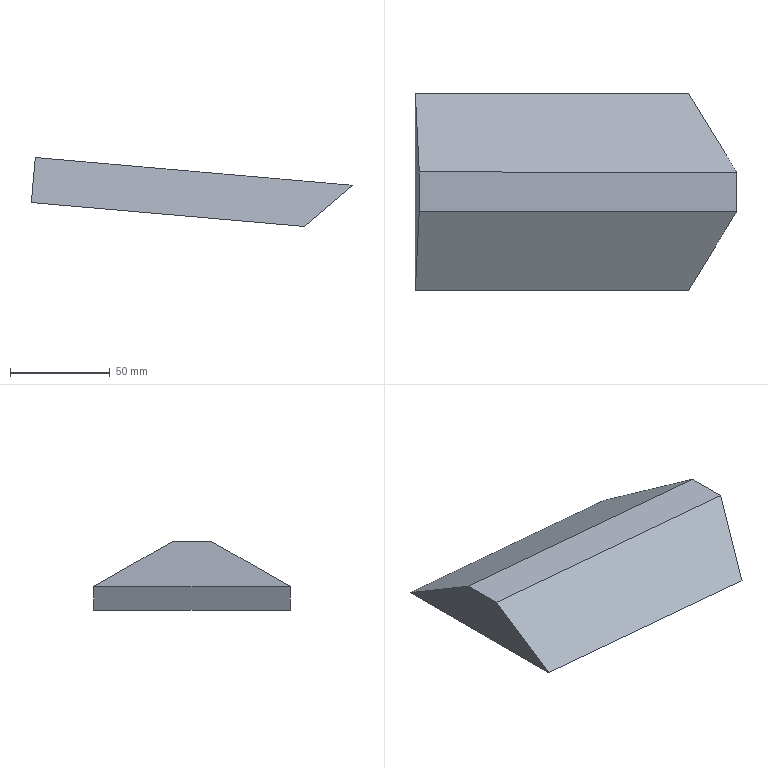Part | NX | features solid 2 | 1 solid | 6 faces | box 161.368 x 98.588 x 34.603 mm | volume 196929 mm3 | plane 6
STEP:
#1=CARTESIAN_POINT('',(-1040.,229.294,-200.));
#2=VERTEX_POINT('',#1);
#3=CARTESIAN_POINT('',(-1040.,130.706,-200.));
#4=VERTEX_POINT('',#3);
#5=CARTESIAN_POINT('',(-1040.,260.,-200.));
#6=DIRECTION('',(0.,-1.,0.));
#7=VECTOR('',#6,1000.);
#8=LINE('',#5,#7);
#9=EDGE_CURVE('',#2,#4,#8,.T.);
#10=ORIENTED_EDGE('',*,*,#9,.T.);
#11=CARTESIAN_POINT('',(-1038.023,170.,-177.4));
#12=VERTEX_POINT('',#11);
#13=CARTESIAN_POINT('',(-1041.545,100.,-217.661));
#14=DIRECTION('',(0.04358,0.866,0.4981));
#15=VECTOR('',#14,1000.);
#16=LINE('',#13,#15);
#17=EDGE_CURVE('',#4,#12,#16,.T.);
#18=ORIENTED_EDGE('',*,*,#17,.T.);
#19=CARTESIAN_POINT('',(-1038.023,190.,-177.4));
#20=VERTEX_POINT('',#19);
#21=CARTESIAN_POINT('',(-1038.023,260.,-177.4));
#22=DIRECTION('',(0.,-1.,0.));
#23=VECTOR('',#22,1000.);
#24=LINE('',#21,#23);
#25=EDGE_CURVE('',#20,#12,#24,.T.);
#26=ORIENTED_EDGE('',*,*,#25,.F.);
#27=CARTESIAN_POINT('',(-1041.545,260.,-217.661));
#28=DIRECTION('',(0.04358,-0.866,0.4981));
#29=VECTOR('',#28,1000.);
#30=LINE('',#27,#29);
#31=EDGE_CURVE('',#2,#20,#30,.T.);
#32=ORIENTED_EDGE('',*,*,#31,.F.);
#33=EDGE_LOOP('',(#10,#18,#26,#32));
#34=FACE_BOUND('',#33,.T.);
#35=CARTESIAN_POINT('',(-1038.023,260.,-177.4));
#36=DIRECTION('',(-0.9962,0.,0.08716));
#37=DIRECTION('',(-0.08716,0.,-0.9962));
#38=AXIS2_PLACEMENT_3D('',#35,#36,#37);
#39=PLANE('',#38);
#40=ADVANCED_FACE('',(#34),#39,.T.);
#41=CARTESIAN_POINT('',(-902.806,130.706,-212.003));
#42=VERTEX_POINT('',#41);
#43=CARTESIAN_POINT('',(-902.806,130.706,-212.003));
#44=DIRECTION('',(0.9962,0.,-0.08716));
#45=VECTOR('',#44,1000.);
#46=LINE('',#43,#45);
#47=EDGE_CURVE('',#4,#42,#46,.T.);
#48=ORIENTED_EDGE('',*,*,#47,.F.);
#49=ORIENTED_EDGE('',*,*,#9,.F.);
#50=CARTESIAN_POINT('',(-902.806,229.294,-212.003));
#51=VERTEX_POINT('',#50);
#52=CARTESIAN_POINT('',(-902.806,229.294,-212.003));
#53=DIRECTION('',(-0.9962,0.,0.08716));
#54=VECTOR('',#53,1000.);
#55=LINE('',#52,#54);
#56=EDGE_CURVE('',#51,#2,#55,.T.);
#57=ORIENTED_EDGE('',*,*,#56,.F.);
#58=CARTESIAN_POINT('',(-902.806,260.,-212.003));
#59=DIRECTION('',(0.,-1.,0.));
#60=VECTOR('',#59,1000.);
#61=LINE('',#58,#60);
#62=EDGE_CURVE('',#51,#42,#61,.T.);
#63=ORIENTED_EDGE('',*,*,#62,.T.);
#64=EDGE_LOOP('',(#48,#49,#57,#63));
#65=FACE_BOUND('',#64,.T.);
#66=CARTESIAN_POINT('',(-902.806,260.,-212.003));
#67=DIRECTION('',(0.08716,0.,0.9962));
#68=DIRECTION('',(-0.9962,0.,0.08716));
#69=AXIS2_PLACEMENT_3D('',#66,#67,#68);
#70=PLANE('',#69);
#71=ADVANCED_FACE('',(#65),#70,.F.);
#72=CARTESIAN_POINT('',(-878.632,170.,-191.345));
#73=VERTEX_POINT('',#72);
#74=CARTESIAN_POINT('',(-845.173,224.384,-162.753));
#75=DIRECTION('',(0.4782,0.7773,0.4087));
#76=VECTOR('',#75,1000.);
#77=LINE('',#74,#76);
#78=EDGE_CURVE('',#42,#73,#77,.T.);
#79=ORIENTED_EDGE('',*,*,#78,.F.);
#80=ORIENTED_EDGE('',*,*,#62,.F.);
#81=CARTESIAN_POINT('',(-878.632,190.,-191.345));
#82=VERTEX_POINT('',#81);
#83=CARTESIAN_POINT('',(-904.655,232.299,-213.583));
#84=DIRECTION('',(-0.4782,0.7773,-0.4087));
#85=VECTOR('',#84,1000.);
#86=LINE('',#83,#85);
#87=EDGE_CURVE('',#82,#51,#86,.T.);
#88=ORIENTED_EDGE('',*,*,#87,.F.);
#89=CARTESIAN_POINT('',(-878.632,260.,-191.345));
#90=DIRECTION('',(0.,-1.,0.));
#91=VECTOR('',#90,1000.);
#92=LINE('',#89,#91);
#93=EDGE_CURVE('',#82,#73,#92,.T.);
#94=ORIENTED_EDGE('',*,*,#93,.T.);
#95=EDGE_LOOP('',(#79,#80,#88,#94));
#96=FACE_BOUND('',#95,.T.);
#97=CARTESIAN_POINT('',(-878.632,260.,-191.345));
#98=DIRECTION('',(-0.6497,0.,0.7602));
#99=DIRECTION('',(-0.7602,0.,-0.6497));
#100=AXIS2_PLACEMENT_3D('',#97,#98,#99);
#101=PLANE('',#100);
#102=ADVANCED_FACE('',(#96),#101,.F.);
#103=ORIENTED_EDGE('',*,*,#25,.T.);
#104=CARTESIAN_POINT('',(-1038.023,170.,-177.4));
#105=DIRECTION('',(0.9962,0.,-0.08716));
#106=VECTOR('',#105,1000.);
#107=LINE('',#104,#106);
#108=EDGE_CURVE('',#12,#73,#107,.T.);
#109=ORIENTED_EDGE('',*,*,#108,.T.);
#110=ORIENTED_EDGE('',*,*,#93,.F.);
#111=CARTESIAN_POINT('',(-1038.023,190.,-177.4));
#112=DIRECTION('',(0.9962,0.,-0.08716));
#113=VECTOR('',#112,1000.);
#114=LINE('',#111,#113);
#115=EDGE_CURVE('',#20,#82,#114,.T.);
#116=ORIENTED_EDGE('',*,*,#115,.F.);
#117=EDGE_LOOP('',(#103,#109,#110,#116));
#118=FACE_BOUND('',#117,.T.);
#119=CARTESIAN_POINT('',(-878.632,260.,-191.345));
#120=DIRECTION('',(0.08716,0.,0.9962));
#121=DIRECTION('',(-0.9962,0.,0.08716));
#122=AXIS2_PLACEMENT_3D('',#119,#120,#121);
#123=PLANE('',#122);
#124=ADVANCED_FACE('',(#118),#123,.T.);
#125=ORIENTED_EDGE('',*,*,#56,.T.);
#126=ORIENTED_EDGE('',*,*,#31,.T.);
#127=ORIENTED_EDGE('',*,*,#115,.T.);
#128=ORIENTED_EDGE('',*,*,#87,.T.);
#129=EDGE_LOOP('',(#125,#126,#127,#128));
#130=FACE_BOUND('',#129,.T.);
#131=CARTESIAN_POINT('',(-1041.545,260.,-217.661));
#132=DIRECTION('',(0.07548,0.5,0.8627));
#133=DIRECTION('',(0.,-0.8652,0.5014));
#134=AXIS2_PLACEMENT_3D('',#131,#132,#133);
#135=PLANE('',#134);
#136=ADVANCED_FACE('',(#130),#135,.T.);
#137=ORIENTED_EDGE('',*,*,#47,.T.);
#138=ORIENTED_EDGE('',*,*,#78,.T.);
#139=ORIENTED_EDGE('',*,*,#108,.F.);
#140=ORIENTED_EDGE('',*,*,#17,.F.);
#141=EDGE_LOOP('',(#137,#138,#139,#140));
#142=FACE_BOUND('',#141,.T.);
#143=CARTESIAN_POINT('',(-1041.545,100.,-217.661));
#144=DIRECTION('',(0.07548,-0.5,0.8627));
#145=DIRECTION('',(0.,0.8652,0.5014));
#146=AXIS2_PLACEMENT_3D('',#143,#144,#145);
#147=PLANE('',#146);
#148=ADVANCED_FACE('',(#142),#147,.T.);
#149=CLOSED_SHELL('',(#40,#71,#102,#124,#136,#148));
#150=MANIFOLD_SOLID_BREP('',#149);
#151=(LENGTH_UNIT()NAMED_UNIT(*)SI_UNIT(.MILLI.,.METRE.));
#152=UNCERTAINTY_MEASURE_WITH_UNIT(LENGTH_MEASURE(0.00001),#151,'','');
#153=(NAMED_UNIT(*)PLANE_ANGLE_UNIT()SI_UNIT($,.RADIAN.));
#154=(NAMED_UNIT(*)SI_UNIT($,.STERADIAN.)SOLID_ANGLE_UNIT());
#155=(GEOMETRIC_REPRESENTATION_CONTEXT(3)GLOBAL_UNCERTAINTY_ASSIGNED_CONTEXT((#152))GLOBAL_UNIT_ASSIGNED_CONTEXT((#151,#153,#154))REPRESENTATION_CONTEXT('',''));
#156=ADVANCED_BREP_SHAPE_REPRESENTATION('',(#150),#155);